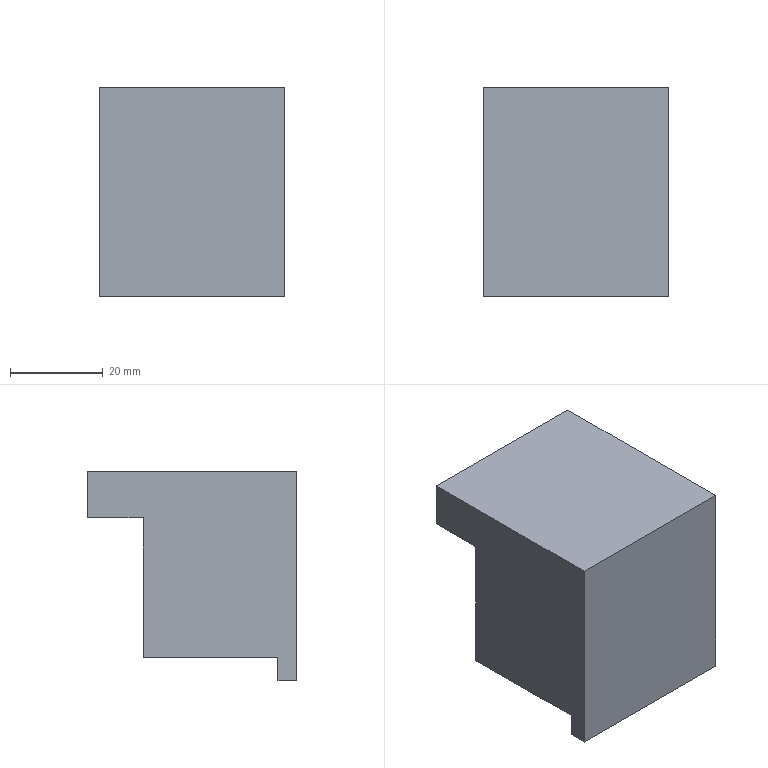Part | NX | features solid 2 | 1 solid | 10 faces | box 40 x 45 x 45 mm | volume 58400 mm3 | plane 10
STEP:
#1=CARTESIAN_POINT('',(-870.,-460.,-120.));
#2=VERTEX_POINT('',#1);
#3=CARTESIAN_POINT('',(-870.,-431.,-120.));
#4=VERTEX_POINT('',#3);
#5=CARTESIAN_POINT('',(-870.,-460.,-120.));
#6=CARTESIAN_POINT('',(-870.,-450.333,-120.));
#7=CARTESIAN_POINT('',(-870.,-440.667,-120.));
#8=CARTESIAN_POINT('',(-870.,-431.,-120.));
#9=B_SPLINE_CURVE_WITH_KNOTS('',3,(#5,#6,#7,#8),.UNSPECIFIED.,.F.,.F.,(4,4),(0.,1.),.UNSPECIFIED.);
#10=EDGE_CURVE('',#2,#4,#9,.T.);
#11=ORIENTED_EDGE('',*,*,#10,.T.);
#12=CARTESIAN_POINT('',(-830.,-431.,-120.));
#13=VERTEX_POINT('',#12);
#14=CARTESIAN_POINT('',(-870.,-431.,-120.));
#15=CARTESIAN_POINT('',(-856.667,-431.,-120.));
#16=CARTESIAN_POINT('',(-843.333,-431.,-120.));
#17=CARTESIAN_POINT('',(-830.,-431.,-120.));
#18=B_SPLINE_CURVE_WITH_KNOTS('',3,(#14,#15,#16,#17),.UNSPECIFIED.,.F.,.F.,(4,4),(0.,1.),.UNSPECIFIED.);
#19=EDGE_CURVE('',#13,#4,#18,.F.);
#20=ORIENTED_EDGE('',*,*,#19,.F.);
#21=CARTESIAN_POINT('',(-830.,-460.,-120.));
#22=VERTEX_POINT('',#21);
#23=CARTESIAN_POINT('',(-830.,-431.,-120.));
#24=CARTESIAN_POINT('',(-830.,-440.667,-120.));
#25=CARTESIAN_POINT('',(-830.,-450.333,-120.));
#26=CARTESIAN_POINT('',(-830.,-460.,-120.));
#27=B_SPLINE_CURVE_WITH_KNOTS('',3,(#23,#24,#25,#26),.UNSPECIFIED.,.F.,.F.,(4,4),(0.,1.),.UNSPECIFIED.);
#28=EDGE_CURVE('',#22,#13,#27,.F.);
#29=ORIENTED_EDGE('',*,*,#28,.F.);
#30=CARTESIAN_POINT('',(-830.,-460.,-120.));
#31=CARTESIAN_POINT('',(-843.333,-460.,-120.));
#32=CARTESIAN_POINT('',(-856.667,-460.,-120.));
#33=CARTESIAN_POINT('',(-870.,-460.,-120.));
#34=B_SPLINE_CURVE_WITH_KNOTS('',3,(#30,#31,#32,#33),.UNSPECIFIED.,.F.,.F.,(4,4),(0.,1.),.UNSPECIFIED.);
#35=EDGE_CURVE('',#22,#2,#34,.T.);
#36=ORIENTED_EDGE('',*,*,#35,.T.);
#37=EDGE_LOOP('',(#11,#20,#29,#36));
#38=FACE_BOUND('',#37,.T.);
#39=CARTESIAN_POINT('',(-830.,-441.5,-120.));
#40=DIRECTION('',(-0.000000341,0.00000017,-1.));
#41=DIRECTION('',(1.,-0.000000011,-0.000000341));
#42=AXIS2_PLACEMENT_3D('',#39,#40,#41);
#43=PLANE('',#42);
#44=ADVANCED_FACE('',(#38),#43,.T.);
#45=CARTESIAN_POINT('',(-870.,-431.,-90.));
#46=VERTEX_POINT('',#45);
#47=CARTESIAN_POINT('',(-870.,-431.,-120.));
#48=CARTESIAN_POINT('',(-870.,-431.,-110.));
#49=CARTESIAN_POINT('',(-870.,-431.,-100.));
#50=CARTESIAN_POINT('',(-870.,-431.,-90.));
#51=B_SPLINE_CURVE_WITH_KNOTS('',3,(#47,#48,#49,#50),.UNSPECIFIED.,.F.,.F.,(4,4),(0.,1.),.UNSPECIFIED.);
#52=EDGE_CURVE('',#4,#46,#51,.T.);
#53=ORIENTED_EDGE('',*,*,#52,.T.);
#54=CARTESIAN_POINT('',(-830.,-431.,-90.));
#55=VERTEX_POINT('',#54);
#56=CARTESIAN_POINT('',(-870.,-431.,-90.));
#57=CARTESIAN_POINT('',(-856.667,-431.,-90.));
#58=CARTESIAN_POINT('',(-843.333,-431.,-90.));
#59=CARTESIAN_POINT('',(-830.,-431.,-90.));
#60=B_SPLINE_CURVE_WITH_KNOTS('',3,(#56,#57,#58,#59),.UNSPECIFIED.,.F.,.F.,(4,4),(0.,1.),.UNSPECIFIED.);
#61=EDGE_CURVE('',#55,#46,#60,.F.);
#62=ORIENTED_EDGE('',*,*,#61,.F.);
#63=CARTESIAN_POINT('',(-830.,-431.,-90.));
#64=CARTESIAN_POINT('',(-830.,-431.,-100.));
#65=CARTESIAN_POINT('',(-830.,-431.,-110.));
#66=CARTESIAN_POINT('',(-830.,-431.,-120.));
#67=B_SPLINE_CURVE_WITH_KNOTS('',3,(#63,#64,#65,#66),.UNSPECIFIED.,.F.,.F.,(4,4),(0.,1.),.UNSPECIFIED.);
#68=EDGE_CURVE('',#13,#55,#67,.F.);
#69=ORIENTED_EDGE('',*,*,#68,.F.);
#70=ORIENTED_EDGE('',*,*,#19,.T.);
#71=EDGE_LOOP('',(#53,#62,#69,#70));
#72=FACE_BOUND('',#71,.T.);
#73=CARTESIAN_POINT('',(-830.,-431.,-102.5));
#74=DIRECTION('',(0.000000011,1.,0.00000017));
#75=DIRECTION('',(0.000000341,-0.00000017,1.));
#76=AXIS2_PLACEMENT_3D('',#73,#74,#75);
#77=PLANE('',#76);
#78=ADVANCED_FACE('',(#72),#77,.T.);
#79=CARTESIAN_POINT('',(-870.,-419.,-90.));
#80=VERTEX_POINT('',#79);
#81=CARTESIAN_POINT('',(-870.,-431.,-90.));
#82=CARTESIAN_POINT('',(-870.,-427.,-90.));
#83=CARTESIAN_POINT('',(-870.,-423.,-90.));
#84=CARTESIAN_POINT('',(-870.,-419.,-90.));
#85=B_SPLINE_CURVE_WITH_KNOTS('',3,(#81,#82,#83,#84),.UNSPECIFIED.,.F.,.F.,(4,4),(0.,1.),.UNSPECIFIED.);
#86=EDGE_CURVE('',#46,#80,#85,.T.);
#87=ORIENTED_EDGE('',*,*,#86,.T.);
#88=CARTESIAN_POINT('',(-830.,-419.,-90.));
#89=VERTEX_POINT('',#88);
#90=CARTESIAN_POINT('',(-870.,-419.,-90.));
#91=CARTESIAN_POINT('',(-856.667,-419.,-90.));
#92=CARTESIAN_POINT('',(-843.333,-419.,-90.));
#93=CARTESIAN_POINT('',(-830.,-419.,-90.));
#94=B_SPLINE_CURVE_WITH_KNOTS('',3,(#90,#91,#92,#93),.UNSPECIFIED.,.F.,.F.,(4,4),(0.,1.),.UNSPECIFIED.);
#95=EDGE_CURVE('',#89,#80,#94,.F.);
#96=ORIENTED_EDGE('',*,*,#95,.F.);
#97=CARTESIAN_POINT('',(-830.,-419.,-90.));
#98=CARTESIAN_POINT('',(-830.,-423.,-90.));
#99=CARTESIAN_POINT('',(-830.,-427.,-90.));
#100=CARTESIAN_POINT('',(-830.,-431.,-90.));
#101=B_SPLINE_CURVE_WITH_KNOTS('',3,(#97,#98,#99,#100),.UNSPECIFIED.,.F.,.F.,(4,4),(0.,1.),.UNSPECIFIED.);
#102=EDGE_CURVE('',#55,#89,#101,.F.);
#103=ORIENTED_EDGE('',*,*,#102,.F.);
#104=ORIENTED_EDGE('',*,*,#61,.T.);
#105=EDGE_LOOP('',(#87,#96,#103,#104));
#106=FACE_BOUND('',#105,.T.);
#107=CARTESIAN_POINT('',(-830.,-441.5,-90.));
#108=DIRECTION('',(-0.000000341,0.00000017,-1.));
#109=DIRECTION('',(1.,-0.000000011,-0.000000341));
#110=AXIS2_PLACEMENT_3D('',#107,#108,#109);
#111=PLANE('',#110);
#112=ADVANCED_FACE('',(#106),#111,.T.);
#113=CARTESIAN_POINT('',(-870.,-419.,-80.));
#114=VERTEX_POINT('',#113);
#115=CARTESIAN_POINT('',(-870.,-419.,-90.));
#116=CARTESIAN_POINT('',(-870.,-419.,-86.666));
#117=CARTESIAN_POINT('',(-870.,-419.,-83.333));
#118=CARTESIAN_POINT('',(-870.,-419.,-80.));
#119=B_SPLINE_CURVE_WITH_KNOTS('',3,(#115,#116,#117,#118),.UNSPECIFIED.,.F.,.F.,(4,4),(0.,1.),.UNSPECIFIED.);
#120=EDGE_CURVE('',#80,#114,#119,.T.);
#121=ORIENTED_EDGE('',*,*,#120,.T.);
#122=CARTESIAN_POINT('',(-830.,-419.,-80.));
#123=VERTEX_POINT('',#122);
#124=CARTESIAN_POINT('',(-870.,-419.,-80.));
#125=CARTESIAN_POINT('',(-856.667,-419.,-80.));
#126=CARTESIAN_POINT('',(-843.333,-419.,-80.));
#127=CARTESIAN_POINT('',(-830.,-419.,-80.));
#128=B_SPLINE_CURVE_WITH_KNOTS('',3,(#124,#125,#126,#127),.UNSPECIFIED.,.F.,.F.,(4,4),(0.,1.),.UNSPECIFIED.);
#129=EDGE_CURVE('',#123,#114,#128,.F.);
#130=ORIENTED_EDGE('',*,*,#129,.F.);
#131=CARTESIAN_POINT('',(-830.,-419.,-80.));
#132=CARTESIAN_POINT('',(-830.,-419.,-83.333));
#133=CARTESIAN_POINT('',(-830.,-419.,-86.666));
#134=CARTESIAN_POINT('',(-830.,-419.,-90.));
#135=B_SPLINE_CURVE_WITH_KNOTS('',3,(#131,#132,#133,#134),.UNSPECIFIED.,.F.,.F.,(4,4),(0.,1.),.UNSPECIFIED.);
#136=EDGE_CURVE('',#89,#123,#135,.F.);
#137=ORIENTED_EDGE('',*,*,#136,.F.);
#138=ORIENTED_EDGE('',*,*,#95,.T.);
#139=EDGE_LOOP('',(#121,#130,#137,#138));
#140=FACE_BOUND('',#139,.T.);
#141=CARTESIAN_POINT('',(-830.,-419.,-102.5));
#142=DIRECTION('',(0.000000011,1.,0.00000017));
#143=DIRECTION('',(0.000000341,-0.00000017,1.));
#144=AXIS2_PLACEMENT_3D('',#141,#142,#143);
#145=PLANE('',#144);
#146=ADVANCED_FACE('',(#140),#145,.T.);
#147=CARTESIAN_POINT('',(-870.,-464.,-80.));
#148=VERTEX_POINT('',#147);
#149=CARTESIAN_POINT('',(-870.,-419.,-80.));
#150=CARTESIAN_POINT('',(-870.,-434.,-80.));
#151=CARTESIAN_POINT('',(-870.,-449.,-80.));
#152=CARTESIAN_POINT('',(-870.,-464.,-80.));
#153=B_SPLINE_CURVE_WITH_KNOTS('',3,(#149,#150,#151,#152),.UNSPECIFIED.,.F.,.F.,(4,4),(0.,1.),.UNSPECIFIED.);
#154=EDGE_CURVE('',#114,#148,#153,.T.);
#155=ORIENTED_EDGE('',*,*,#154,.T.);
#156=CARTESIAN_POINT('',(-830.,-464.,-80.));
#157=VERTEX_POINT('',#156);
#158=CARTESIAN_POINT('',(-870.,-464.,-80.));
#159=CARTESIAN_POINT('',(-856.667,-464.,-80.));
#160=CARTESIAN_POINT('',(-843.333,-464.,-80.));
#161=CARTESIAN_POINT('',(-830.,-464.,-80.));
#162=B_SPLINE_CURVE_WITH_KNOTS('',3,(#158,#159,#160,#161),.UNSPECIFIED.,.F.,.F.,(4,4),(0.,1.),.UNSPECIFIED.);
#163=EDGE_CURVE('',#157,#148,#162,.F.);
#164=ORIENTED_EDGE('',*,*,#163,.F.);
#165=CARTESIAN_POINT('',(-830.,-464.,-80.));
#166=CARTESIAN_POINT('',(-830.,-449.,-80.));
#167=CARTESIAN_POINT('',(-830.,-434.,-80.));
#168=CARTESIAN_POINT('',(-830.,-419.,-80.));
#169=B_SPLINE_CURVE_WITH_KNOTS('',3,(#165,#166,#167,#168),.UNSPECIFIED.,.F.,.F.,(4,4),(0.,1.),.UNSPECIFIED.);
#170=EDGE_CURVE('',#123,#157,#169,.F.);
#171=ORIENTED_EDGE('',*,*,#170,.F.);
#172=ORIENTED_EDGE('',*,*,#129,.T.);
#173=EDGE_LOOP('',(#155,#164,#171,#172));
#174=FACE_BOUND('',#173,.T.);
#175=CARTESIAN_POINT('',(-830.,-441.5,-80.));
#176=DIRECTION('',(0.000000341,-0.00000017,1.));
#177=DIRECTION('',(-1.,0.000000011,0.000000341));
#178=AXIS2_PLACEMENT_3D('',#175,#176,#177);
#179=PLANE('',#178);
#180=ADVANCED_FACE('',(#174),#179,.T.);
#181=CARTESIAN_POINT('',(-870.,-464.,-125.));
#182=VERTEX_POINT('',#181);
#183=CARTESIAN_POINT('',(-870.,-464.,-80.));
#184=CARTESIAN_POINT('',(-870.,-464.,-95.));
#185=CARTESIAN_POINT('',(-870.,-464.,-110.));
#186=CARTESIAN_POINT('',(-870.,-464.,-125.));
#187=B_SPLINE_CURVE_WITH_KNOTS('',3,(#183,#184,#185,#186),.UNSPECIFIED.,.F.,.F.,(4,4),(0.,1.),.UNSPECIFIED.);
#188=EDGE_CURVE('',#148,#182,#187,.T.);
#189=ORIENTED_EDGE('',*,*,#188,.T.);
#190=CARTESIAN_POINT('',(-830.,-464.,-125.));
#191=VERTEX_POINT('',#190);
#192=CARTESIAN_POINT('',(-870.,-464.,-125.));
#193=CARTESIAN_POINT('',(-856.667,-464.,-125.));
#194=CARTESIAN_POINT('',(-843.333,-464.,-125.));
#195=CARTESIAN_POINT('',(-830.,-464.,-125.));
#196=B_SPLINE_CURVE_WITH_KNOTS('',3,(#192,#193,#194,#195),.UNSPECIFIED.,.F.,.F.,(4,4),(0.,1.),.UNSPECIFIED.);
#197=EDGE_CURVE('',#191,#182,#196,.F.);
#198=ORIENTED_EDGE('',*,*,#197,.F.);
#199=CARTESIAN_POINT('',(-830.,-464.,-125.));
#200=CARTESIAN_POINT('',(-830.,-464.,-110.));
#201=CARTESIAN_POINT('',(-830.,-464.,-95.));
#202=CARTESIAN_POINT('',(-830.,-464.,-80.));
#203=B_SPLINE_CURVE_WITH_KNOTS('',3,(#199,#200,#201,#202),.UNSPECIFIED.,.F.,.F.,(4,4),(0.,1.),.UNSPECIFIED.);
#204=EDGE_CURVE('',#157,#191,#203,.F.);
#205=ORIENTED_EDGE('',*,*,#204,.F.);
#206=ORIENTED_EDGE('',*,*,#163,.T.);
#207=EDGE_LOOP('',(#189,#198,#205,#206));
#208=FACE_BOUND('',#207,.T.);
#209=CARTESIAN_POINT('',(-830.,-464.,-102.5));
#210=DIRECTION('',(-0.000000011,-1.,-0.00000017));
#211=DIRECTION('',(-0.000000341,0.00000017,-1.));
#212=AXIS2_PLACEMENT_3D('',#209,#210,#211);
#213=PLANE('',#212);
#214=ADVANCED_FACE('',(#208),#213,.T.);
#215=CARTESIAN_POINT('',(-870.,-460.,-125.));
#216=VERTEX_POINT('',#215);
#217=CARTESIAN_POINT('',(-870.,-464.,-125.));
#218=CARTESIAN_POINT('',(-870.,-462.667,-125.));
#219=CARTESIAN_POINT('',(-870.,-461.333,-125.));
#220=CARTESIAN_POINT('',(-870.,-460.,-125.));
#221=B_SPLINE_CURVE_WITH_KNOTS('',3,(#217,#218,#219,#220),.UNSPECIFIED.,.F.,.F.,(4,4),(0.,1.),.UNSPECIFIED.);
#222=EDGE_CURVE('',#182,#216,#221,.T.);
#223=ORIENTED_EDGE('',*,*,#222,.T.);
#224=CARTESIAN_POINT('',(-830.,-460.,-125.));
#225=VERTEX_POINT('',#224);
#226=CARTESIAN_POINT('',(-870.,-460.,-125.));
#227=CARTESIAN_POINT('',(-856.667,-460.,-125.));
#228=CARTESIAN_POINT('',(-843.333,-460.,-125.));
#229=CARTESIAN_POINT('',(-830.,-460.,-125.));
#230=B_SPLINE_CURVE_WITH_KNOTS('',3,(#226,#227,#228,#229),.UNSPECIFIED.,.F.,.F.,(4,4),(0.,1.),.UNSPECIFIED.);
#231=EDGE_CURVE('',#225,#216,#230,.F.);
#232=ORIENTED_EDGE('',*,*,#231,.F.);
#233=CARTESIAN_POINT('',(-830.,-460.,-125.));
#234=CARTESIAN_POINT('',(-830.,-461.333,-125.));
#235=CARTESIAN_POINT('',(-830.,-462.667,-125.));
#236=CARTESIAN_POINT('',(-830.,-464.,-125.));
#237=B_SPLINE_CURVE_WITH_KNOTS('',3,(#233,#234,#235,#236),.UNSPECIFIED.,.F.,.F.,(4,4),(0.,1.),.UNSPECIFIED.);
#238=EDGE_CURVE('',#191,#225,#237,.F.);
#239=ORIENTED_EDGE('',*,*,#238,.F.);
#240=ORIENTED_EDGE('',*,*,#197,.T.);
#241=EDGE_LOOP('',(#223,#232,#239,#240));
#242=FACE_BOUND('',#241,.T.);
#243=CARTESIAN_POINT('',(-830.,-441.5,-125.));
#244=DIRECTION('',(-0.000000341,0.00000017,-1.));
#245=DIRECTION('',(1.,-0.000000011,-0.000000341));
#246=AXIS2_PLACEMENT_3D('',#243,#244,#245);
#247=PLANE('',#246);
#248=ADVANCED_FACE('',(#242),#247,.T.);
#249=CARTESIAN_POINT('',(-870.,-460.,-125.));
#250=CARTESIAN_POINT('',(-870.,-460.,-123.333));
#251=CARTESIAN_POINT('',(-870.,-460.,-121.666));
#252=CARTESIAN_POINT('',(-870.,-460.,-120.));
#253=B_SPLINE_CURVE_WITH_KNOTS('',3,(#249,#250,#251,#252),.UNSPECIFIED.,.F.,.F.,(4,4),(0.,1.),.UNSPECIFIED.);
#254=EDGE_CURVE('',#216,#2,#253,.T.);
#255=ORIENTED_EDGE('',*,*,#254,.T.);
#256=ORIENTED_EDGE('',*,*,#35,.F.);
#257=CARTESIAN_POINT('',(-830.,-460.,-120.));
#258=CARTESIAN_POINT('',(-830.,-460.,-121.666));
#259=CARTESIAN_POINT('',(-830.,-460.,-123.333));
#260=CARTESIAN_POINT('',(-830.,-460.,-125.));
#261=B_SPLINE_CURVE_WITH_KNOTS('',3,(#257,#258,#259,#260),.UNSPECIFIED.,.F.,.F.,(4,4),(0.,1.),.UNSPECIFIED.);
#262=EDGE_CURVE('',#225,#22,#261,.F.);
#263=ORIENTED_EDGE('',*,*,#262,.F.);
#264=ORIENTED_EDGE('',*,*,#231,.T.);
#265=EDGE_LOOP('',(#255,#256,#263,#264));
#266=FACE_BOUND('',#265,.T.);
#267=CARTESIAN_POINT('',(-830.,-460.,-102.5));
#268=DIRECTION('',(0.000000011,1.,0.00000017));
#269=DIRECTION('',(0.000000341,-0.00000017,1.));
#270=AXIS2_PLACEMENT_3D('',#267,#268,#269);
#271=PLANE('',#270);
#272=ADVANCED_FACE('',(#266),#271,.T.);
#273=ORIENTED_EDGE('',*,*,#28,.T.);
#274=ORIENTED_EDGE('',*,*,#68,.T.);
#275=ORIENTED_EDGE('',*,*,#102,.T.);
#276=ORIENTED_EDGE('',*,*,#136,.T.);
#277=ORIENTED_EDGE('',*,*,#170,.T.);
#278=ORIENTED_EDGE('',*,*,#204,.T.);
#279=ORIENTED_EDGE('',*,*,#238,.T.);
#280=ORIENTED_EDGE('',*,*,#262,.T.);
#281=EDGE_LOOP('',(#273,#274,#275,#276,#277,#278,#279,#280));
#282=FACE_BOUND('',#281,.T.);
#283=CARTESIAN_POINT('',(-830.,-441.5,-102.5));
#284=DIRECTION('',(-1.,0.000000011,0.000000341));
#285=DIRECTION('',(0.000000011,1.,0.00000017));
#286=AXIS2_PLACEMENT_3D('',#283,#284,#285);
#287=PLANE('',#286);
#288=ADVANCED_FACE('',(#282),#287,.F.);
#289=ORIENTED_EDGE('',*,*,#10,.F.);
#290=ORIENTED_EDGE('',*,*,#254,.F.);
#291=ORIENTED_EDGE('',*,*,#222,.F.);
#292=ORIENTED_EDGE('',*,*,#188,.F.);
#293=ORIENTED_EDGE('',*,*,#154,.F.);
#294=ORIENTED_EDGE('',*,*,#120,.F.);
#295=ORIENTED_EDGE('',*,*,#86,.F.);
#296=ORIENTED_EDGE('',*,*,#52,.F.);
#297=EDGE_LOOP('',(#289,#290,#291,#292,#293,#294,#295,#296));
#298=FACE_BOUND('',#297,.T.);
#299=CARTESIAN_POINT('',(-870.,-441.5,-102.5));
#300=DIRECTION('',(-1.,0.000000011,0.000000341));
#301=DIRECTION('',(0.000000011,1.,0.00000017));
#302=AXIS2_PLACEMENT_3D('',#299,#300,#301);
#303=PLANE('',#302);
#304=ADVANCED_FACE('',(#298),#303,.T.);
#305=CLOSED_SHELL('',(#44,#78,#112,#146,#180,#214,#248,#272,#288,#304));
#306=MANIFOLD_SOLID_BREP('',#305);
#307=(LENGTH_UNIT()NAMED_UNIT(*)SI_UNIT(.MILLI.,.METRE.));
#308=UNCERTAINTY_MEASURE_WITH_UNIT(LENGTH_MEASURE(0.0508),#307,'','');
#309=(NAMED_UNIT(*)PLANE_ANGLE_UNIT()SI_UNIT($,.RADIAN.));
#310=(NAMED_UNIT(*)SI_UNIT($,.STERADIAN.)SOLID_ANGLE_UNIT());
#311=(GEOMETRIC_REPRESENTATION_CONTEXT(3)GLOBAL_UNCERTAINTY_ASSIGNED_CONTEXT((#308))GLOBAL_UNIT_ASSIGNED_CONTEXT((#307,#309,#310))REPRESENTATION_CONTEXT('',''));
#312=ADVANCED_BREP_SHAPE_REPRESENTATION('',(#306),#311);